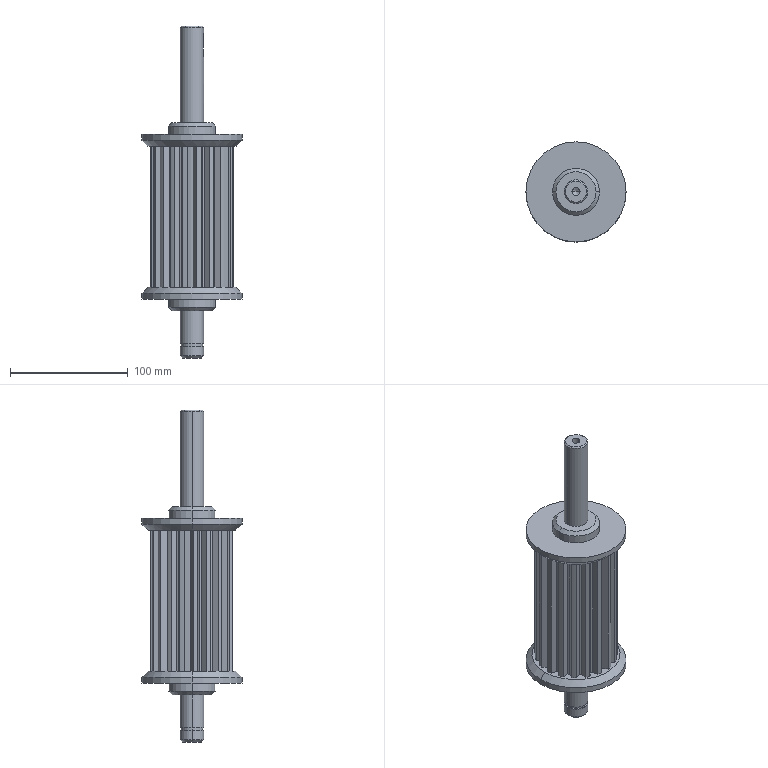Part | STEP file | Driven roller | 1 solid | 125 faces | box 85 x 85 x 282 mm | volume 574522 mm3 | cylinder 60 | plane 51 | cone 14 | commonest cylinder face diameters 60 x19 70 x19 20 x6 6 x4 40 x4 85 x4